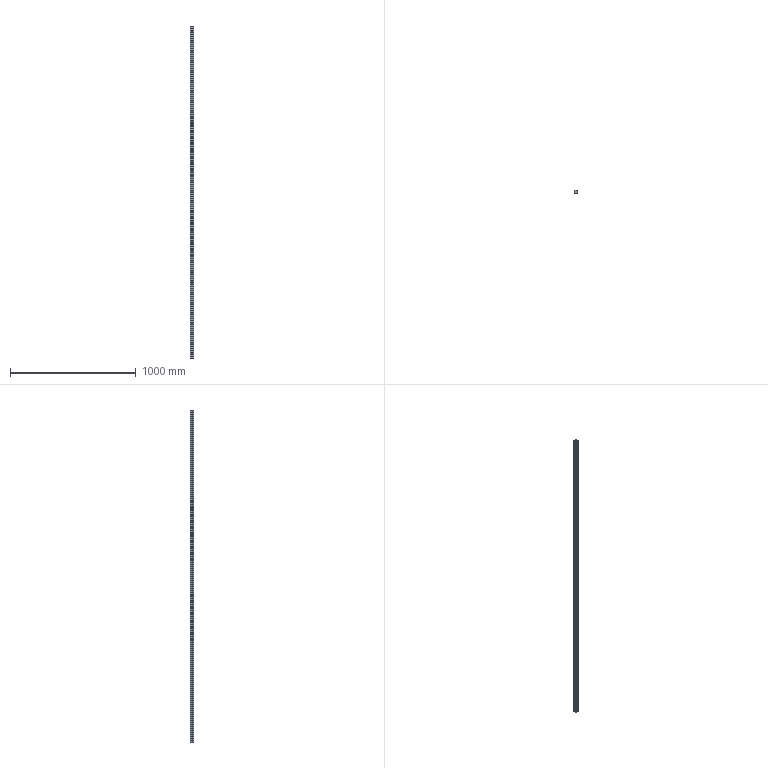Part | SolidWorks | features BaseBody 1 | 1 solid | 348 faces | box 28 x 26 x 2640 mm | volume 1534033 mm3 | cylinder 162 | plane 129 | spline 57 | commonest cylinder face diameters 9 x66 14 x66 1.2 x20 1.6 x6 5.66 x4